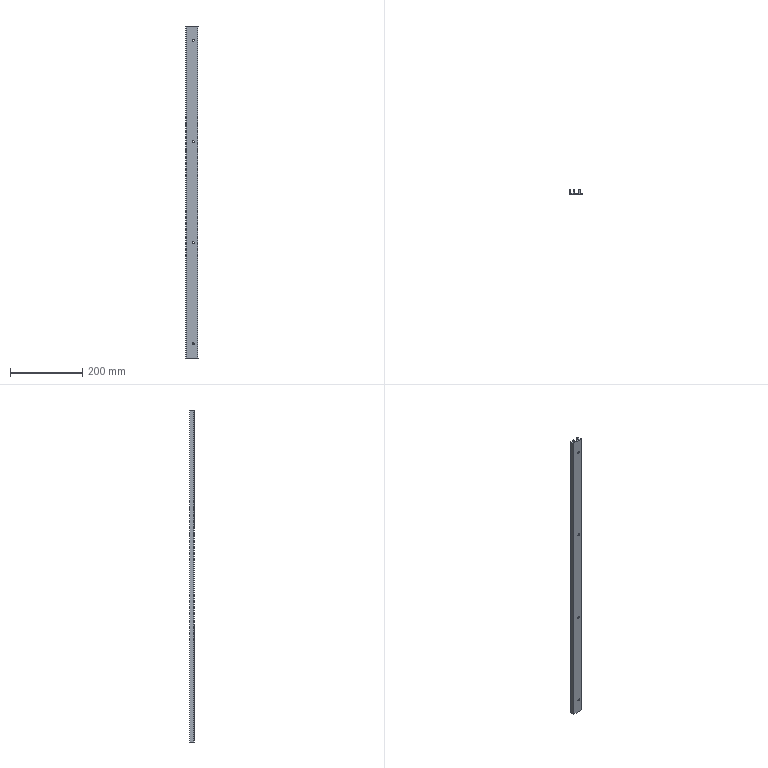Part | NX | features BREP 1 | 1 solid | 41 faces | box 33.5 x 13.5 x 919.5 mm | volume 171516 mm3 | cylinder 17 | plane 16 | cone 8 | commonest cylinder face diameters 5.5 x8 10.6 x4 4 x2 1.5 x1 2.5 x1 3 x1
STEP:
#1=CARTESIAN_POINT('',(22.75,0.45,-420.25));
#2=VERTEX_POINT('',#1);
#3=CARTESIAN_POINT('',(17.25,0.45,-420.25));
#4=VERTEX_POINT('',#3);
#5=CARTESIAN_POINT('',(20.,0.45,-420.25));
#6=DIRECTION('',(0.,1.,0.));
#7=DIRECTION('',(-1.,0.,0.));
#8=AXIS2_PLACEMENT_3D('',#5,#6,#7);
#9=CIRCLE('',#8,2.75);
#10=EDGE_CURVE('',#2,#4,#9,.T.);
#11=ORIENTED_EDGE('',*,*,#10,.F.);
#12=CARTESIAN_POINT('',(25.3,3.,-420.25));
#13=VERTEX_POINT('',#12);
#14=CARTESIAN_POINT('',(25.3,3.,-420.25));
#15=DIRECTION('',(0.7071,0.7071,0.));
#16=VECTOR('',#15,1000.);
#17=LINE('',#14,#16);
#18=EDGE_CURVE('',#2,#13,#17,.T.);
#19=ORIENTED_EDGE('',*,*,#18,.T.);
#20=CARTESIAN_POINT('',(24.5,3.,-423.05));
#21=VERTEX_POINT('',#20);
#22=CARTESIAN_POINT('',(20.,3.,-420.25));
#23=DIRECTION('',(0.,1.,0.));
#24=DIRECTION('',(-1.,0.,0.));
#25=AXIS2_PLACEMENT_3D('',#22,#23,#24);
#26=CIRCLE('',#25,5.3);
#27=EDGE_CURVE('',#13,#21,#26,.T.);
#28=ORIENTED_EDGE('',*,*,#27,.T.);
#29=CARTESIAN_POINT('',(14.7,3.,-420.25));
#30=VERTEX_POINT('',#29);
#31=CARTESIAN_POINT('',(20.,3.,-420.25));
#32=DIRECTION('',(0.,-1.,0.));
#33=DIRECTION('',(1.,0.,0.));
#34=AXIS2_PLACEMENT_3D('',#31,#32,#33);
#35=CIRCLE('',#34,5.3);
#36=EDGE_CURVE('',#30,#21,#35,.T.);
#37=ORIENTED_EDGE('',*,*,#36,.F.);
#38=CARTESIAN_POINT('',(14.7,3.,-420.25));
#39=DIRECTION('',(-0.7071,0.7071,0.));
#40=VECTOR('',#39,1000.);
#41=LINE('',#38,#40);
#42=EDGE_CURVE('',#4,#30,#41,.T.);
#43=ORIENTED_EDGE('',*,*,#42,.F.);
#44=EDGE_LOOP('',(#11,#19,#28,#37,#43));
#45=FACE_BOUND('',#44,.T.);
#46=CARTESIAN_POINT('',(20.,3.,-420.25));
#47=DIRECTION('',(0.,1.,0.));
#48=DIRECTION('',(-1.,0.,0.));
#49=AXIS2_PLACEMENT_3D('',#46,#47,#48);
#50=CONICAL_SURFACE('',#49,5.3,0.7854);
#51=ADVANCED_FACE('',(#45),#50,.F.);
#52=CARTESIAN_POINT('',(22.75,0.,-420.25));
#53=VERTEX_POINT('',#52);
#54=CARTESIAN_POINT('',(17.25,0.,-420.25));
#55=VERTEX_POINT('',#54);
#56=CARTESIAN_POINT('',(20.,0.,-420.25));
#57=DIRECTION('',(0.,1.,0.));
#58=DIRECTION('',(-1.,0.,0.));
#59=AXIS2_PLACEMENT_3D('',#56,#57,#58);
#60=CIRCLE('',#59,2.75);
#61=EDGE_CURVE('',#53,#55,#60,.T.);
#62=ORIENTED_EDGE('',*,*,#61,.F.);
#63=CARTESIAN_POINT('',(22.75,12.402,-420.25));
#64=DIRECTION('',(0.,1.,0.));
#65=VECTOR('',#64,1000.);
#66=LINE('',#63,#65);
#67=EDGE_CURVE('',#53,#2,#66,.T.);
#68=ORIENTED_EDGE('',*,*,#67,.T.);
#69=ORIENTED_EDGE('',*,*,#10,.T.);
#70=CARTESIAN_POINT('',(17.25,12.402,-420.25));
#71=DIRECTION('',(0.,1.,0.));
#72=VECTOR('',#71,1000.);
#73=LINE('',#70,#72);
#74=EDGE_CURVE('',#55,#4,#73,.T.);
#75=ORIENTED_EDGE('',*,*,#74,.F.);
#76=EDGE_LOOP('',(#62,#68,#69,#75));
#77=FACE_BOUND('',#76,.T.);
#78=CARTESIAN_POINT('',(20.,12.402,-420.25));
#79=DIRECTION('',(0.,1.,0.));
#80=DIRECTION('',(-1.,0.,0.));
#81=AXIS2_PLACEMENT_3D('',#78,#79,#80);
#82=CYLINDRICAL_SURFACE('',#81,2.75);
#83=ADVANCED_FACE('',(#77),#82,.F.);
#84=CARTESIAN_POINT('',(22.75,0.45,-140.25));
#85=VERTEX_POINT('',#84);
#86=CARTESIAN_POINT('',(17.25,0.45,-140.25));
#87=VERTEX_POINT('',#86);
#88=CARTESIAN_POINT('',(20.,0.45,-140.25));
#89=DIRECTION('',(0.,1.,0.));
#90=DIRECTION('',(-1.,0.,0.));
#91=AXIS2_PLACEMENT_3D('',#88,#89,#90);
#92=CIRCLE('',#91,2.75);
#93=EDGE_CURVE('',#85,#87,#92,.T.);
#94=ORIENTED_EDGE('',*,*,#93,.F.);
#95=CARTESIAN_POINT('',(25.3,3.,-140.25));
#96=VERTEX_POINT('',#95);
#97=CARTESIAN_POINT('',(25.3,3.,-140.25));
#98=DIRECTION('',(0.7071,0.7071,0.));
#99=VECTOR('',#98,1000.);
#100=LINE('',#97,#99);
#101=EDGE_CURVE('',#85,#96,#100,.T.);
#102=ORIENTED_EDGE('',*,*,#101,.T.);
#103=CARTESIAN_POINT('',(24.5,3.,-143.05));
#104=VERTEX_POINT('',#103);
#105=CARTESIAN_POINT('',(20.,3.,-140.25));
#106=DIRECTION('',(0.,1.,0.));
#107=DIRECTION('',(-1.,0.,0.));
#108=AXIS2_PLACEMENT_3D('',#105,#106,#107);
#109=CIRCLE('',#108,5.3);
#110=EDGE_CURVE('',#96,#104,#109,.T.);
#111=ORIENTED_EDGE('',*,*,#110,.T.);
#112=CARTESIAN_POINT('',(14.7,3.,-140.25));
#113=VERTEX_POINT('',#112);
#114=CARTESIAN_POINT('',(20.,3.,-140.25));
#115=DIRECTION('',(0.,-1.,0.));
#116=DIRECTION('',(1.,0.,0.));
#117=AXIS2_PLACEMENT_3D('',#114,#115,#116);
#118=CIRCLE('',#117,5.3);
#119=EDGE_CURVE('',#113,#104,#118,.T.);
#120=ORIENTED_EDGE('',*,*,#119,.F.);
#121=CARTESIAN_POINT('',(14.7,3.,-140.25));
#122=DIRECTION('',(-0.7071,0.7071,0.));
#123=VECTOR('',#122,1000.);
#124=LINE('',#121,#123);
#125=EDGE_CURVE('',#87,#113,#124,.T.);
#126=ORIENTED_EDGE('',*,*,#125,.F.);
#127=EDGE_LOOP('',(#94,#102,#111,#120,#126));
#128=FACE_BOUND('',#127,.T.);
#129=CARTESIAN_POINT('',(20.,3.,-140.25));
#130=DIRECTION('',(0.,1.,0.));
#131=DIRECTION('',(-1.,0.,0.));
#132=AXIS2_PLACEMENT_3D('',#129,#130,#131);
#133=CONICAL_SURFACE('',#132,5.3,0.7854);
#134=ADVANCED_FACE('',(#128),#133,.F.);
#135=CARTESIAN_POINT('',(22.75,0.,-140.25));
#136=VERTEX_POINT('',#135);
#137=CARTESIAN_POINT('',(17.25,0.,-140.25));
#138=VERTEX_POINT('',#137);
#139=CARTESIAN_POINT('',(20.,0.,-140.25));
#140=DIRECTION('',(0.,1.,0.));
#141=DIRECTION('',(-1.,0.,0.));
#142=AXIS2_PLACEMENT_3D('',#139,#140,#141);
#143=CIRCLE('',#142,2.75);
#144=EDGE_CURVE('',#136,#138,#143,.T.);
#145=ORIENTED_EDGE('',*,*,#144,.F.);
#146=CARTESIAN_POINT('',(22.75,12.402,-140.25));
#147=DIRECTION('',(0.,1.,0.));
#148=VECTOR('',#147,1000.);
#149=LINE('',#146,#148);
#150=EDGE_CURVE('',#136,#85,#149,.T.);
#151=ORIENTED_EDGE('',*,*,#150,.T.);
#152=ORIENTED_EDGE('',*,*,#93,.T.);
#153=CARTESIAN_POINT('',(17.25,12.402,-140.25));
#154=DIRECTION('',(0.,1.,0.));
#155=VECTOR('',#154,1000.);
#156=LINE('',#153,#155);
#157=EDGE_CURVE('',#138,#87,#156,.T.);
#158=ORIENTED_EDGE('',*,*,#157,.F.);
#159=EDGE_LOOP('',(#145,#151,#152,#158));
#160=FACE_BOUND('',#159,.T.);
#161=CARTESIAN_POINT('',(20.,12.402,-140.25));
#162=DIRECTION('',(0.,1.,0.));
#163=DIRECTION('',(-1.,0.,0.));
#164=AXIS2_PLACEMENT_3D('',#161,#162,#163);
#165=CYLINDRICAL_SURFACE('',#164,2.75);
#166=ADVANCED_FACE('',(#160),#165,.F.);
#167=CARTESIAN_POINT('',(22.75,0.45,139.75));
#168=VERTEX_POINT('',#167);
#169=CARTESIAN_POINT('',(17.25,0.45,139.75));
#170=VERTEX_POINT('',#169);
#171=CARTESIAN_POINT('',(20.,0.45,139.75));
#172=DIRECTION('',(0.,1.,0.));
#173=DIRECTION('',(-1.,0.,0.));
#174=AXIS2_PLACEMENT_3D('',#171,#172,#173);
#175=CIRCLE('',#174,2.75);
#176=EDGE_CURVE('',#168,#170,#175,.T.);
#177=ORIENTED_EDGE('',*,*,#176,.F.);
#178=CARTESIAN_POINT('',(25.3,3.,139.75));
#179=VERTEX_POINT('',#178);
#180=CARTESIAN_POINT('',(25.3,3.,139.75));
#181=DIRECTION('',(0.7071,0.7071,0.));
#182=VECTOR('',#181,1000.);
#183=LINE('',#180,#182);
#184=EDGE_CURVE('',#168,#179,#183,.T.);
#185=ORIENTED_EDGE('',*,*,#184,.T.);
#186=CARTESIAN_POINT('',(24.5,3.,136.95));
#187=VERTEX_POINT('',#186);
#188=CARTESIAN_POINT('',(20.,3.,139.75));
#189=DIRECTION('',(0.,1.,0.));
#190=DIRECTION('',(-1.,0.,0.));
#191=AXIS2_PLACEMENT_3D('',#188,#189,#190);
#192=CIRCLE('',#191,5.3);
#193=EDGE_CURVE('',#179,#187,#192,.T.);
#194=ORIENTED_EDGE('',*,*,#193,.T.);
#195=CARTESIAN_POINT('',(14.7,3.,139.75));
#196=VERTEX_POINT('',#195);
#197=CARTESIAN_POINT('',(20.,3.,139.75));
#198=DIRECTION('',(0.,-1.,0.));
#199=DIRECTION('',(1.,0.,0.));
#200=AXIS2_PLACEMENT_3D('',#197,#198,#199);
#201=CIRCLE('',#200,5.3);
#202=EDGE_CURVE('',#196,#187,#201,.T.);
#203=ORIENTED_EDGE('',*,*,#202,.F.);
#204=CARTESIAN_POINT('',(14.7,3.,139.75));
#205=DIRECTION('',(-0.7071,0.7071,0.));
#206=VECTOR('',#205,1000.);
#207=LINE('',#204,#206);
#208=EDGE_CURVE('',#170,#196,#207,.T.);
#209=ORIENTED_EDGE('',*,*,#208,.F.);
#210=EDGE_LOOP('',(#177,#185,#194,#203,#209));
#211=FACE_BOUND('',#210,.T.);
#212=CARTESIAN_POINT('',(20.,3.,139.75));
#213=DIRECTION('',(0.,1.,0.));
#214=DIRECTION('',(-1.,0.,0.));
#215=AXIS2_PLACEMENT_3D('',#212,#213,#214);
#216=CONICAL_SURFACE('',#215,5.3,0.7854);
#217=ADVANCED_FACE('',(#211),#216,.F.);
#218=CARTESIAN_POINT('',(22.75,0.,139.75));
#219=VERTEX_POINT('',#218);
#220=CARTESIAN_POINT('',(17.25,0.,139.75));
#221=VERTEX_POINT('',#220);
#222=CARTESIAN_POINT('',(20.,0.,139.75));
#223=DIRECTION('',(0.,1.,0.));
#224=DIRECTION('',(-1.,0.,0.));
#225=AXIS2_PLACEMENT_3D('',#222,#223,#224);
#226=CIRCLE('',#225,2.75);
#227=EDGE_CURVE('',#219,#221,#226,.T.);
#228=ORIENTED_EDGE('',*,*,#227,.F.);
#229=CARTESIAN_POINT('',(22.75,12.402,139.75));
#230=DIRECTION('',(0.,1.,0.));
#231=VECTOR('',#230,1000.);
#232=LINE('',#229,#231);
#233=EDGE_CURVE('',#219,#168,#232,.T.);
#234=ORIENTED_EDGE('',*,*,#233,.T.);
#235=ORIENTED_EDGE('',*,*,#176,.T.);
#236=CARTESIAN_POINT('',(17.25,12.402,139.75));
#237=DIRECTION('',(0.,1.,0.));
#238=VECTOR('',#237,1000.);
#239=LINE('',#236,#238);
#240=EDGE_CURVE('',#221,#170,#239,.T.);
#241=ORIENTED_EDGE('',*,*,#240,.F.);
#242=EDGE_LOOP('',(#228,#234,#235,#241));
#243=FACE_BOUND('',#242,.T.);
#244=CARTESIAN_POINT('',(20.,12.402,139.75));
#245=DIRECTION('',(0.,1.,0.));
#246=DIRECTION('',(-1.,0.,0.));
#247=AXIS2_PLACEMENT_3D('',#244,#245,#246);
#248=CYLINDRICAL_SURFACE('',#247,2.75);
#249=ADVANCED_FACE('',(#243),#248,.F.);
#250=CARTESIAN_POINT('',(22.75,0.45,419.75));
#251=VERTEX_POINT('',#250);
#252=CARTESIAN_POINT('',(17.25,0.45,419.75));
#253=VERTEX_POINT('',#252);
#254=CARTESIAN_POINT('',(20.,0.45,419.75));
#255=DIRECTION('',(0.,1.,0.));
#256=DIRECTION('',(-1.,0.,0.));
#257=AXIS2_PLACEMENT_3D('',#254,#255,#256);
#258=CIRCLE('',#257,2.75);
#259=EDGE_CURVE('',#251,#253,#258,.T.);
#260=ORIENTED_EDGE('',*,*,#259,.F.);
#261=CARTESIAN_POINT('',(25.3,3.,419.75));
#262=VERTEX_POINT('',#261);
#263=CARTESIAN_POINT('',(25.3,3.,419.75));
#264=DIRECTION('',(0.7071,0.7071,0.));
#265=VECTOR('',#264,1000.);
#266=LINE('',#263,#265);
#267=EDGE_CURVE('',#251,#262,#266,.T.);
#268=ORIENTED_EDGE('',*,*,#267,.T.);
#269=CARTESIAN_POINT('',(24.5,3.,416.95));
#270=VERTEX_POINT('',#269);
#271=CARTESIAN_POINT('',(20.,3.,419.75));
#272=DIRECTION('',(0.,1.,0.));
#273=DIRECTION('',(-1.,0.,0.));
#274=AXIS2_PLACEMENT_3D('',#271,#272,#273);
#275=CIRCLE('',#274,5.3);
#276=EDGE_CURVE('',#262,#270,#275,.T.);
#277=ORIENTED_EDGE('',*,*,#276,.T.);
#278=CARTESIAN_POINT('',(14.7,3.,419.75));
#279=VERTEX_POINT('',#278);
#280=CARTESIAN_POINT('',(20.,3.,419.75));
#281=DIRECTION('',(0.,-1.,0.));
#282=DIRECTION('',(1.,0.,0.));
#283=AXIS2_PLACEMENT_3D('',#280,#281,#282);
#284=CIRCLE('',#283,5.3);
#285=EDGE_CURVE('',#279,#270,#284,.T.);
#286=ORIENTED_EDGE('',*,*,#285,.F.);
#287=CARTESIAN_POINT('',(14.7,3.,419.75));
#288=DIRECTION('',(-0.7071,0.7071,0.));
#289=VECTOR('',#288,1000.);
#290=LINE('',#287,#289);
#291=EDGE_CURVE('',#253,#279,#290,.T.);
#292=ORIENTED_EDGE('',*,*,#291,.F.);
#293=EDGE_LOOP('',(#260,#268,#277,#286,#292));
#294=FACE_BOUND('',#293,.T.);
#295=CARTESIAN_POINT('',(20.,3.,419.75));
#296=DIRECTION('',(0.,1.,0.));
#297=DIRECTION('',(-1.,0.,0.));
#298=AXIS2_PLACEMENT_3D('',#295,#296,#297);
#299=CONICAL_SURFACE('',#298,5.3,0.7854);
#300=ADVANCED_FACE('',(#294),#299,.F.);
#301=CARTESIAN_POINT('',(22.75,0.,419.75));
#302=VERTEX_POINT('',#301);
#303=CARTESIAN_POINT('',(17.25,0.,419.75));
#304=VERTEX_POINT('',#303);
#305=CARTESIAN_POINT('',(20.,0.,419.75));
#306=DIRECTION('',(0.,1.,0.));
#307=DIRECTION('',(-1.,0.,0.));
#308=AXIS2_PLACEMENT_3D('',#305,#306,#307);
#309=CIRCLE('',#308,2.75);
#310=EDGE_CURVE('',#302,#304,#309,.T.);
#311=ORIENTED_EDGE('',*,*,#310,.F.);
#312=CARTESIAN_POINT('',(22.75,12.402,419.75));
#313=DIRECTION('',(0.,1.,0.));
#314=VECTOR('',#313,1000.);
#315=LINE('',#312,#314);
#316=EDGE_CURVE('',#302,#251,#315,.T.);
#317=ORIENTED_EDGE('',*,*,#316,.T.);
#318=ORIENTED_EDGE('',*,*,#259,.T.);
#319=CARTESIAN_POINT('',(17.25,12.402,419.75));
#320=DIRECTION('',(0.,1.,0.));
#321=VECTOR('',#320,1000.);
#322=LINE('',#319,#321);
#323=EDGE_CURVE('',#304,#253,#322,.T.);
#324=ORIENTED_EDGE('',*,*,#323,.F.);
#325=EDGE_LOOP('',(#311,#317,#318,#324));
#326=FACE_BOUND('',#325,.T.);
#327=CARTESIAN_POINT('',(20.,12.402,419.75));
#328=DIRECTION('',(0.,1.,0.));
#329=DIRECTION('',(-1.,0.,0.));
#330=AXIS2_PLACEMENT_3D('',#327,#328,#329);
#331=CYLINDRICAL_SURFACE('',#330,2.75);
#332=ADVANCED_FACE('',(#326),#331,.F.);
#333=CARTESIAN_POINT('',(24.5,3.,-459.75));
#334=VERTEX_POINT('',#333);
#335=CARTESIAN_POINT('',(24.5,3.,459.75));
#336=DIRECTION('',(0.,0.,-1.));
#337=VECTOR('',#336,1000.);
#338=LINE('',#335,#337);
#339=EDGE_CURVE('',#21,#334,#338,.T.);
#340=ORIENTED_EDGE('',*,*,#339,.F.);
#341=CARTESIAN_POINT('',(24.5,10.5,-423.05));
#342=VERTEX_POINT('',#341);
#343=CARTESIAN_POINT('',(24.5,12.402,-423.05));
#344=DIRECTION('',(0.,1.,0.));
#345=VECTOR('',#344,1000.);
#346=LINE('',#343,#345);
#347=EDGE_CURVE('',#21,#342,#346,.T.);
#348=ORIENTED_EDGE('',*,*,#347,.T.);
#349=CARTESIAN_POINT('',(24.5,10.5,-459.75));
#350=VERTEX_POINT('',#349);
#351=CARTESIAN_POINT('',(24.5,10.5,459.75));
#352=DIRECTION('',(0.,0.,-1.));
#353=VECTOR('',#352,1000.);
#354=LINE('',#351,#353);
#355=EDGE_CURVE('',#342,#350,#354,.T.);
#356=ORIENTED_EDGE('',*,*,#355,.T.);
#357=CARTESIAN_POINT('',(24.5,3.,-459.75));
#358=DIRECTION('',(0.,-1.,0.));
#359=VECTOR('',#358,1000.);
#360=LINE('',#357,#359);
#361=EDGE_CURVE('',#350,#334,#360,.T.);
#362=ORIENTED_EDGE('',*,*,#361,.T.);
#363=EDGE_LOOP('',(#340,#348,#356,#362));
#364=FACE_BOUND('',#363,.T.);
#365=CARTESIAN_POINT('',(24.5,3.,459.75));
#366=DIRECTION('',(1.,0.,0.));
#367=DIRECTION('',(0.,1.,0.));
#368=AXIS2_PLACEMENT_3D('',#365,#366,#367);
#369=PLANE('',#368);
#370=ADVANCED_FACE('',(#364),#369,.F.);
#371=CARTESIAN_POINT('',(24.5,10.5,-143.05));
#372=VERTEX_POINT('',#371);
#373=CARTESIAN_POINT('',(24.5,10.5,-417.45));
#374=VERTEX_POINT('',#373);
#375=CARTESIAN_POINT('',(24.5,10.5,459.75));
#376=DIRECTION('',(0.,0.,-1.));
#377=VECTOR('',#376,1000.);
#378=LINE('',#375,#377);
#379=EDGE_CURVE('',#372,#374,#378,.T.);
#380=ORIENTED_EDGE('',*,*,#379,.T.);
#381=CARTESIAN_POINT('',(24.5,3.,-417.45));
#382=VERTEX_POINT('',#381);
#383=CARTESIAN_POINT('',(24.5,12.402,-417.45));
#384=DIRECTION('',(0.,-1.,0.));
#385=VECTOR('',#384,1000.);
#386=LINE('',#383,#385);
#387=EDGE_CURVE('',#374,#382,#386,.T.);
#388=ORIENTED_EDGE('',*,*,#387,.T.);
#389=CARTESIAN_POINT('',(24.5,3.,459.75));
#390=DIRECTION('',(0.,0.,-1.));
#391=VECTOR('',#390,1000.);
#392=LINE('',#389,#391);
#393=EDGE_CURVE('',#104,#382,#392,.T.);
#394=ORIENTED_EDGE('',*,*,#393,.F.);
#395=CARTESIAN_POINT('',(24.5,12.402,-143.05));
#396=DIRECTION('',(0.,1.,0.));
#397=VECTOR('',#396,1000.);
#398=LINE('',#395,#397);
#399=EDGE_CURVE('',#104,#372,#398,.T.);
#400=ORIENTED_EDGE('',*,*,#399,.T.);
#401=EDGE_LOOP('',(#380,#388,#394,#400));
#402=FACE_BOUND('',#401,.T.);
#403=CARTESIAN_POINT('',(24.5,3.,459.75));
#404=DIRECTION('',(1.,0.,0.));
#405=DIRECTION('',(0.,1.,0.));
#406=AXIS2_PLACEMENT_3D('',#403,#404,#405);
#407=PLANE('',#406);
#408=ADVANCED_FACE('',(#402),#407,.F.);
#409=CARTESIAN_POINT('',(24.5,10.5,136.95));
#410=VERTEX_POINT('',#409);
#411=CARTESIAN_POINT('',(24.5,10.5,-137.45));
#412=VERTEX_POINT('',#411);
#413=CARTESIAN_POINT('',(24.5,10.5,459.75));
#414=DIRECTION('',(0.,0.,-1.));
#415=VECTOR('',#414,1000.);
#416=LINE('',#413,#415);
#417=EDGE_CURVE('',#410,#412,#416,.T.);
#418=ORIENTED_EDGE('',*,*,#417,.T.);
#419=CARTESIAN_POINT('',(24.5,3.,-137.45));
#420=VERTEX_POINT('',#419);
#421=CARTESIAN_POINT('',(24.5,12.402,-137.45));
#422=DIRECTION('',(0.,-1.,0.));
#423=VECTOR('',#422,1000.);
#424=LINE('',#421,#423);
#425=EDGE_CURVE('',#412,#420,#424,.T.);
#426=ORIENTED_EDGE('',*,*,#425,.T.);
#427=CARTESIAN_POINT('',(24.5,3.,459.75));
#428=DIRECTION('',(0.,0.,-1.));
#429=VECTOR('',#428,1000.);
#430=LINE('',#427,#429);
#431=EDGE_CURVE('',#187,#420,#430,.T.);
#432=ORIENTED_EDGE('',*,*,#431,.F.);
#433=CARTESIAN_POINT('',(24.5,12.402,136.95));
#434=DIRECTION('',(0.,1.,0.));
#435=VECTOR('',#434,1000.);
#436=LINE('',#433,#435);
#437=EDGE_CURVE('',#187,#410,#436,.T.);
#438=ORIENTED_EDGE('',*,*,#437,.T.);
#439=EDGE_LOOP('',(#418,#426,#432,#438));
#440=FACE_BOUND('',#439,.T.);
#441=CARTESIAN_POINT('',(24.5,3.,459.75));
#442=DIRECTION('',(1.,0.,0.));
#443=DIRECTION('',(0.,1.,0.));
#444=AXIS2_PLACEMENT_3D('',#441,#442,#443);
#445=PLANE('',#444);
#446=ADVANCED_FACE('',(#440),#445,.F.);
#447=CARTESIAN_POINT('',(24.5,10.5,416.95));
#448=VERTEX_POINT('',#447);
#449=CARTESIAN_POINT('',(24.5,10.5,142.55));
#450=VERTEX_POINT('',#449);
#451=CARTESIAN_POINT('',(24.5,10.5,459.75));
#452=DIRECTION('',(0.,0.,-1.));
#453=VECTOR('',#452,1000.);
#454=LINE('',#451,#453);
#455=EDGE_CURVE('',#448,#450,#454,.T.);
#456=ORIENTED_EDGE('',*,*,#455,.T.);
#457=CARTESIAN_POINT('',(24.5,3.,142.55));
#458=VERTEX_POINT('',#457);
#459=CARTESIAN_POINT('',(24.5,12.402,142.55));
#460=DIRECTION('',(0.,-1.,0.));
#461=VECTOR('',#460,1000.);
#462=LINE('',#459,#461);
#463=EDGE_CURVE('',#450,#458,#462,.T.);
#464=ORIENTED_EDGE('',*,*,#463,.T.);
#465=CARTESIAN_POINT('',(24.5,3.,459.75));
#466=DIRECTION('',(0.,0.,-1.));
#467=VECTOR('',#466,1000.);
#468=LINE('',#465,#467);
#469=EDGE_CURVE('',#270,#458,#468,.T.);
#470=ORIENTED_EDGE('',*,*,#469,.F.);
#471=CARTESIAN_POINT('',(24.5,12.402,416.95));
#472=DIRECTION('',(0.,1.,0.));
#473=VECTOR('',#472,1000.);
#474=LINE('',#471,#473);
#475=EDGE_CURVE('',#270,#448,#474,.T.);
#476=ORIENTED_EDGE('',*,*,#475,.T.);
#477=EDGE_LOOP('',(#456,#464,#470,#476));
#478=FACE_BOUND('',#477,.T.);
#479=CARTESIAN_POINT('',(24.5,3.,459.75));
#480=DIRECTION('',(1.,0.,0.));
#481=DIRECTION('',(0.,1.,0.));
#482=AXIS2_PLACEMENT_3D('',#479,#480,#481);
#483=PLANE('',#482);
#484=ADVANCED_FACE('',(#478),#483,.F.);
#485=CARTESIAN_POINT('',(0.,1.25,-459.75));
#486=VERTEX_POINT('',#485);
#487=CARTESIAN_POINT('',(1.25,0.,-459.75));
#488=VERTEX_POINT('',#487);
#489=CARTESIAN_POINT('',(1.25,1.25,-459.75));
#490=DIRECTION('',(0.,0.,1.));
#491=DIRECTION('',(1.,0.,0.));
#492=AXIS2_PLACEMENT_3D('',#489,#490,#491);
#493=CIRCLE('',#492,1.25);
#494=EDGE_CURVE('',#486,#488,#493,.T.);
#495=ORIENTED_EDGE('',*,*,#494,.T.);
#496=CARTESIAN_POINT('',(1.25,0.,459.75));
#497=VERTEX_POINT('',#496);
#498=CARTESIAN_POINT('',(1.25,0.,459.75));
#499=DIRECTION('',(0.,0.,-1.));
#500=VECTOR('',#499,1000.);
#501=LINE('',#498,#500);
#502=EDGE_CURVE('',#497,#488,#501,.T.);
#503=ORIENTED_EDGE('',*,*,#502,.F.);
#504=CARTESIAN_POINT('',(0.,1.25,459.75));
#505=VERTEX_POINT('',#504);
#506=CARTESIAN_POINT('',(1.25,1.25,459.75));
#507=DIRECTION('',(0.,0.,1.));
#508=DIRECTION('',(1.,0.,0.));
#509=AXIS2_PLACEMENT_3D('',#506,#507,#508);
#510=CIRCLE('',#509,1.25);
#511=EDGE_CURVE('',#505,#497,#510,.T.);
#512=ORIENTED_EDGE('',*,*,#511,.F.);
#513=CARTESIAN_POINT('',(0.,1.25,459.75));
#514=DIRECTION('',(0.,0.,-1.));
#515=VECTOR('',#514,1000.);
#516=LINE('',#513,#515);
#517=EDGE_CURVE('',#505,#486,#516,.T.);
#518=ORIENTED_EDGE('',*,*,#517,.T.);
#519=EDGE_LOOP('',(#495,#503,#512,#518));
#520=FACE_BOUND('',#519,.T.);
#521=CARTESIAN_POINT('',(1.25,1.25,459.75));
#522=DIRECTION('',(0.,0.,-1.));
#523=DIRECTION('',(-1.,0.,0.));
#524=AXIS2_PLACEMENT_3D('',#521,#522,#523);
#525=CYLINDRICAL_SURFACE('',#524,1.25);
#526=ADVANCED_FACE('',(#520),#525,.T.);
#527=CARTESIAN_POINT('',(32.,0.,-459.75));
#528=VERTEX_POINT('',#527);
#529=CARTESIAN_POINT('',(1.25,0.,-459.75));
#530=DIRECTION('',(1.,0.,0.));
#531=VECTOR('',#530,1000.);
#532=LINE('',#529,#531);
#533=EDGE_CURVE('',#488,#528,#532,.T.);
#534=ORIENTED_EDGE('',*,*,#533,.T.);
#535=CARTESIAN_POINT('',(32.,0.,459.75));
#536=VERTEX_POINT('',#535);
#537=CARTESIAN_POINT('',(32.,0.,459.75));
#538=DIRECTION('',(0.,0.,-1.));
#539=VECTOR('',#538,1000.);
#540=LINE('',#537,#539);
#541=EDGE_CURVE('',#536,#528,#540,.T.);
#542=ORIENTED_EDGE('',*,*,#541,.F.);
#543=CARTESIAN_POINT('',(1.25,0.,459.75));
#544=DIRECTION('',(1.,0.,0.));
#545=VECTOR('',#544,1000.);
#546=LINE('',#543,#545);
#547=EDGE_CURVE('',#497,#536,#546,.T.);
#548=ORIENTED_EDGE('',*,*,#547,.F.);
#549=ORIENTED_EDGE('',*,*,#502,.T.);
#550=EDGE_LOOP('',(#534,#542,#548,#549));
#551=FACE_BOUND('',#550,.T.);
#552=CARTESIAN_POINT('',(20.,0.,-420.25));
#553=DIRECTION('',(0.,1.,0.));
#554=DIRECTION('',(-1.,0.,0.));
#555=AXIS2_PLACEMENT_3D('',#552,#553,#554);
#556=CIRCLE('',#555,2.75);
#557=EDGE_CURVE('',#55,#53,#556,.T.);
#558=ORIENTED_EDGE('',*,*,#557,.T.);
#559=ORIENTED_EDGE('',*,*,#61,.T.);
#560=EDGE_LOOP('',(#558,#559));
#561=FACE_BOUND('',#560,.T.);
#562=CARTESIAN_POINT('',(20.,0.,-140.25));
#563=DIRECTION('',(0.,1.,0.));
#564=DIRECTION('',(-1.,0.,0.));
#565=AXIS2_PLACEMENT_3D('',#562,#563,#564);
#566=CIRCLE('',#565,2.75);
#567=EDGE_CURVE('',#138,#136,#566,.T.);
#568=ORIENTED_EDGE('',*,*,#567,.T.);
#569=ORIENTED_EDGE('',*,*,#144,.T.);
#570=EDGE_LOOP('',(#568,#569));
#571=FACE_BOUND('',#570,.T.);
#572=CARTESIAN_POINT('',(20.,0.,139.75));
#573=DIRECTION('',(0.,1.,0.));
#574=DIRECTION('',(-1.,0.,0.));
#575=AXIS2_PLACEMENT_3D('',#572,#573,#574);
#576=CIRCLE('',#575,2.75);
#577=EDGE_CURVE('',#221,#219,#576,.T.);
#578=ORIENTED_EDGE('',*,*,#577,.T.);
#579=ORIENTED_EDGE('',*,*,#227,.T.);
#580=EDGE_LOOP('',(#578,#579));
#581=FACE_BOUND('',#580,.T.);
#582=CARTESIAN_POINT('',(20.,0.,419.75));
#583=DIRECTION('',(0.,1.,0.));
#584=DIRECTION('',(-1.,0.,0.));
#585=AXIS2_PLACEMENT_3D('',#582,#583,#584);
#586=CIRCLE('',#585,2.75);
#587=EDGE_CURVE('',#304,#302,#586,.T.);
#588=ORIENTED_EDGE('',*,*,#587,.T.);
#589=ORIENTED_EDGE('',*,*,#310,.T.);
#590=EDGE_LOOP('',(#588,#589));
#591=FACE_BOUND('',#590,.T.);
#592=CARTESIAN_POINT('',(1.25,0.,459.75));
#593=DIRECTION('',(0.,1.,0.));
#594=DIRECTION('',(1.,0.,0.));
#595=AXIS2_PLACEMENT_3D('',#592,#593,#594);
#596=PLANE('',#595);
#597=ADVANCED_FACE('',(#551,#561,#571,#581,#591),#596,.F.);
#598=CARTESIAN_POINT('',(32.,3.,-459.75));
#599=VERTEX_POINT('',#598);
#600=CARTESIAN_POINT('',(32.,1.5,-459.75));
#601=DIRECTION('',(0.,0.,1.));
#602=DIRECTION('',(-1.,0.,0.));
#603=AXIS2_PLACEMENT_3D('',#600,#601,#602);
#604=CIRCLE('',#603,1.5);
#605=EDGE_CURVE('',#528,#599,#604,.T.);
#606=ORIENTED_EDGE('',*,*,#605,.T.);
#607=CARTESIAN_POINT('',(32.,3.,459.75));
#608=VERTEX_POINT('',#607);
#609=CARTESIAN_POINT('',(32.,3.,459.75));
#610=DIRECTION('',(0.,0.,-1.));
#611=VECTOR('',#610,1000.);
#612=LINE('',#609,#611);
#613=EDGE_CURVE('',#608,#599,#612,.T.);
#614=ORIENTED_EDGE('',*,*,#613,.F.);
#615=CARTESIAN_POINT('',(32.,1.5,459.75));
#616=DIRECTION('',(0.,0.,1.));
#617=DIRECTION('',(-1.,0.,0.));
#618=AXIS2_PLACEMENT_3D('',#615,#616,#617);
#619=CIRCLE('',#618,1.5);
#620=EDGE_CURVE('',#536,#608,#619,.T.);
#621=ORIENTED_EDGE('',*,*,#620,.F.);
#622=ORIENTED_EDGE('',*,*,#541,.T.);
#623=EDGE_LOOP('',(#606,#614,#621,#622));
#624=FACE_BOUND('',#623,.T.);
#625=CARTESIAN_POINT('',(32.,1.5,459.75));
#626=DIRECTION('',(0.,0.,-1.));
#627=DIRECTION('',(-1.,0.,0.));
#628=AXIS2_PLACEMENT_3D('',#625,#626,#627);
#629=CYLINDRICAL_SURFACE('',#628,1.5);
#630=ADVANCED_FACE('',(#624),#629,.T.);
#631=CARTESIAN_POINT('',(28.5,3.,-459.75));
#632=VERTEX_POINT('',#631);
#633=CARTESIAN_POINT('',(28.5,3.,-459.75));
#634=DIRECTION('',(-1.,0.,0.));
#635=VECTOR('',#634,1000.);
#636=LINE('',#633,#635);
#637=EDGE_CURVE('',#599,#632,#636,.T.);
#638=ORIENTED_EDGE('',*,*,#637,.T.);
#639=CARTESIAN_POINT('',(28.5,3.,459.75));
#640=VERTEX_POINT('',#639);
#641=CARTESIAN_POINT('',(28.5,3.,459.75));
#642=DIRECTION('',(0.,0.,-1.));
#643=VECTOR('',#642,1000.);
#644=LINE('',#641,#643);
#645=EDGE_CURVE('',#640,#632,#644,.T.);
#646=ORIENTED_EDGE('',*,*,#645,.F.);
#647=CARTESIAN_POINT('',(28.5,3.,459.75));
#648=DIRECTION('',(-1.,0.,0.));
#649=VECTOR('',#648,1000.);
#650=LINE('',#647,#649);
#651=EDGE_CURVE('',#608,#640,#650,.T.);
#652=ORIENTED_EDGE('',*,*,#651,.F.);
#653=ORIENTED_EDGE('',*,*,#613,.T.);
#654=EDGE_LOOP('',(#638,#646,#652,#653));
#655=FACE_BOUND('',#654,.T.);
#656=CARTESIAN_POINT('',(28.5,3.,459.75));
#657=DIRECTION('',(0.,-1.,0.));
#658=DIRECTION('',(0.,0.,-1.));
#659=AXIS2_PLACEMENT_3D('',#656,#657,#658);
#660=PLANE('',#659);
#661=ADVANCED_FACE('',(#655),#660,.F.);
#662=CARTESIAN_POINT('',(28.5,10.5,-459.75));
#663=VERTEX_POINT('',#662);
#664=CARTESIAN_POINT('',(28.5,10.5,-459.75));
#665=DIRECTION('',(0.,1.,0.));
#666=VECTOR('',#665,1000.);
#667=LINE('',#664,#666);
#668=EDGE_CURVE('',#632,#663,#667,.T.);
#669=ORIENTED_EDGE('',*,*,#668,.T.);
#670=CARTESIAN_POINT('',(28.5,10.5,459.75));
#671=VERTEX_POINT('',#670);
#672=CARTESIAN_POINT('',(28.5,10.5,459.75));
#673=DIRECTION('',(0.,0.,-1.));
#674=VECTOR('',#673,1000.);
#675=LINE('',#672,#674);
#676=EDGE_CURVE('',#671,#663,#675,.T.);
#677=ORIENTED_EDGE('',*,*,#676,.F.);
#678=CARTESIAN_POINT('',(28.5,10.5,459.75));
#679=DIRECTION('',(0.,1.,0.));
#680=VECTOR('',#679,1000.);
#681=LINE('',#678,#680);
#682=EDGE_CURVE('',#640,#671,#681,.T.);
#683=ORIENTED_EDGE('',*,*,#682,.F.);
#684=ORIENTED_EDGE('',*,*,#645,.T.);
#685=EDGE_LOOP('',(#669,#677,#683,#684));
#686=FACE_BOUND('',#685,.T.);
#687=CARTESIAN_POINT('',(28.5,10.5,459.75));
#688=DIRECTION('',(-1.,0.,0.));
#689=DIRECTION('',(0.,0.,1.));
#690=AXIS2_PLACEMENT_3D('',#687,#688,#689);
#691=PLANE('',#690);
#692=ADVANCED_FACE('',(#686),#691,.F.);
#693=ORIENTED_EDGE('',*,*,#355,.F.);
#694=CARTESIAN_POINT('',(24.5,10.5,-423.05));
#695=CARTESIAN_POINT('',(24.5,10.807,-423.05));
#696=CARTESIAN_POINT('',(24.662,11.403,-422.801));
#697=CARTESIAN_POINT('',(25.131,12.006,-421.793));
#698=CARTESIAN_POINT('',(25.412,12.162,-420.25));
#699=CARTESIAN_POINT('',(25.133,12.008,-418.711));
#700=CARTESIAN_POINT('',(24.662,11.404,-417.699));
#701=CARTESIAN_POINT('',(24.5,10.808,-417.45));
#702=CARTESIAN_POINT('',(24.5,10.5,-417.45));
#703=B_SPLINE_CURVE_WITH_KNOTS('',3,(#694,#695,#696,#697,#698,#699,#700,#701,#702),.UNSPECIFIED.,.F.,.F.,(4,1,1,1,1,1,4),(0.,0.125,0.25,0.5,0.75,0.875,1.),.UNSPECIFIED.);
#704=EDGE_CURVE('',#342,#374,#703,.T.);
#705=ORIENTED_EDGE('',*,*,#704,.T.);
#706=ORIENTED_EDGE('',*,*,#379,.F.);
#707=CARTESIAN_POINT('',(24.5,10.5,-143.05));
#708=CARTESIAN_POINT('',(24.5,10.807,-143.05));
#709=CARTESIAN_POINT('',(24.662,11.403,-142.801));
#710=CARTESIAN_POINT('',(25.131,12.006,-141.793));
#711=CARTESIAN_POINT('',(25.412,12.162,-140.25));
#712=CARTESIAN_POINT('',(25.133,12.008,-138.711));
#713=CARTESIAN_POINT('',(24.662,11.404,-137.699));
#714=CARTESIAN_POINT('',(24.5,10.808,-137.45));
#715=CARTESIAN_POINT('',(24.5,10.5,-137.45));
#716=B_SPLINE_CURVE_WITH_KNOTS('',3,(#707,#708,#709,#710,#711,#712,#713,#714,#715),.UNSPECIFIED.,.F.,.F.,(4,1,1,1,1,1,4),(0.,0.125,0.25,0.5,0.75,0.875,1.),.UNSPECIFIED.);
#717=EDGE_CURVE('',#372,#412,#716,.T.);
#718=ORIENTED_EDGE('',*,*,#717,.T.);
#719=ORIENTED_EDGE('',*,*,#417,.F.);
#720=CARTESIAN_POINT('',(24.5,10.5,136.95));
#721=CARTESIAN_POINT('',(24.5,10.807,136.95));
#722=CARTESIAN_POINT('',(24.662,11.403,137.199));
#723=CARTESIAN_POINT('',(25.131,12.006,138.207));
#724=CARTESIAN_POINT('',(25.412,12.162,139.75));
#725=CARTESIAN_POINT('',(25.133,12.008,141.289));
#726=CARTESIAN_POINT('',(24.662,11.404,142.301));
#727=CARTESIAN_POINT('',(24.5,10.808,142.55));
#728=CARTESIAN_POINT('',(24.5,10.5,142.55));
#729=B_SPLINE_CURVE_WITH_KNOTS('',3,(#720,#721,#722,#723,#724,#725,#726,#727,#728),.UNSPECIFIED.,.F.,.F.,(4,1,1,1,1,1,4),(0.,0.125,0.25,0.5,0.75,0.875,1.),.UNSPECIFIED.);
#730=EDGE_CURVE('',#410,#450,#729,.T.);
#731=ORIENTED_EDGE('',*,*,#730,.T.);
#732=ORIENTED_EDGE('',*,*,#455,.F.);
#733=CARTESIAN_POINT('',(24.5,10.5,422.55));
#734=VERTEX_POINT('',#733);
#735=CARTESIAN_POINT('',(24.5,10.5,416.95));
#736=CARTESIAN_POINT('',(24.5,10.807,416.95));
#737=CARTESIAN_POINT('',(24.662,11.403,417.199));
#738=CARTESIAN_POINT('',(25.131,12.006,418.207));
#739=CARTESIAN_POINT('',(25.412,12.162,419.75));
#740=CARTESIAN_POINT('',(25.133,12.008,421.289));
#741=CARTESIAN_POINT('',(24.662,11.404,422.301));
#742=CARTESIAN_POINT('',(24.5,10.808,422.55));
#743=CARTESIAN_POINT('',(24.5,10.5,422.55));
#744=B_SPLINE_CURVE_WITH_KNOTS('',3,(#735,#736,#737,#738,#739,#740,#741,#742,#743),.UNSPECIFIED.,.F.,.F.,(4,1,1,1,1,1,4),(0.,0.125,0.25,0.5,0.75,0.875,1.),.UNSPECIFIED.);
#745=EDGE_CURVE('',#448,#734,#744,.T.);
#746=ORIENTED_EDGE('',*,*,#745,.T.);
#747=CARTESIAN_POINT('',(24.5,10.5,459.75));
#748=VERTEX_POINT('',#747);
#749=CARTESIAN_POINT('',(24.5,10.5,459.75));
#750=DIRECTION('',(0.,0.,-1.));
#751=VECTOR('',#750,1000.);
#752=LINE('',#749,#751);
#753=EDGE_CURVE('',#748,#734,#752,.T.);
#754=ORIENTED_EDGE('',*,*,#753,.F.);
#755=CARTESIAN_POINT('',(26.5,10.5,459.75));
#756=DIRECTION('',(0.,0.,1.));
#757=DIRECTION('',(-1.,0.,0.));
#758=AXIS2_PLACEMENT_3D('',#755,#756,#757);
#759=CIRCLE('',#758,2.);
#760=EDGE_CURVE('',#671,#748,#759,.T.);
#761=ORIENTED_EDGE('',*,*,#760,.F.);
#762=ORIENTED_EDGE('',*,*,#676,.T.);
#763=CARTESIAN_POINT('',(26.5,10.5,-459.75));
#764=DIRECTION('',(0.,0.,1.));
#765=DIRECTION('',(-1.,0.,0.));
#766=AXIS2_PLACEMENT_3D('',#763,#764,#765);
#767=CIRCLE('',#766,2.);
#768=EDGE_CURVE('',#663,#350,#767,.T.);
#769=ORIENTED_EDGE('',*,*,#768,.T.);
#770=EDGE_LOOP('',(#693,#705,#706,#718,#719,#731,#732,#746,#754,#761,#762,#769));
#771=FACE_BOUND('',#770,.T.);
#772=CARTESIAN_POINT('',(26.5,10.5,459.75));
#773=DIRECTION('',(0.,0.,-1.));
#774=DIRECTION('',(-1.,0.,0.));
#775=AXIS2_PLACEMENT_3D('',#772,#773,#774);
#776=CYLINDRICAL_SURFACE('',#775,2.);
#777=ADVANCED_FACE('',(#771),#776,.T.);
#778=ORIENTED_EDGE('',*,*,#753,.T.);
#779=CARTESIAN_POINT('',(24.5,3.,422.55));
#780=VERTEX_POINT('',#779);
#781=CARTESIAN_POINT('',(24.5,12.402,422.55));
#782=DIRECTION('',(0.,-1.,0.));
#783=VECTOR('',#782,1000.);
#784=LINE('',#781,#783);
#785=EDGE_CURVE('',#734,#780,#784,.T.);
#786=ORIENTED_EDGE('',*,*,#785,.T.);
#787=CARTESIAN_POINT('',(24.5,3.,459.75));
#788=VERTEX_POINT('',#787);
#789=CARTESIAN_POINT('',(24.5,3.,459.75));
#790=DIRECTION('',(0.,0.,-1.));
#791=VECTOR('',#790,1000.);
#792=LINE('',#789,#791);
#793=EDGE_CURVE('',#788,#780,#792,.T.);
#794=ORIENTED_EDGE('',*,*,#793,.F.);
#795=CARTESIAN_POINT('',(24.5,3.,459.75));
#796=DIRECTION('',(0.,-1.,0.));
#797=VECTOR('',#796,1000.);
#798=LINE('',#795,#797);
#799=EDGE_CURVE('',#748,#788,#798,.T.);
#800=ORIENTED_EDGE('',*,*,#799,.F.);
#801=EDGE_LOOP('',(#778,#786,#794,#800));
#802=FACE_BOUND('',#801,.T.);
#803=CARTESIAN_POINT('',(24.5,3.,459.75));
#804=DIRECTION('',(1.,0.,0.));
#805=DIRECTION('',(0.,1.,0.));
#806=AXIS2_PLACEMENT_3D('',#803,#804,#805);
#807=PLANE('',#806);
#808=ADVANCED_FACE('',(#802),#807,.F.);
#809=ORIENTED_EDGE('',*,*,#393,.T.);
#810=CARTESIAN_POINT('',(20.,3.,-420.25));
#811=DIRECTION('',(0.,-1.,0.));
#812=DIRECTION('',(1.,0.,0.));
#813=AXIS2_PLACEMENT_3D('',#810,#811,#812);
#814=CIRCLE('',#813,5.3);
#815=EDGE_CURVE('',#382,#30,#814,.T.);
#816=ORIENTED_EDGE('',*,*,#815,.T.);
#817=ORIENTED_EDGE('',*,*,#36,.T.);
#818=ORIENTED_EDGE('',*,*,#339,.T.);
#819=CARTESIAN_POINT('',(12.5,3.,-459.75));
#820=VERTEX_POINT('',#819);
#821=CARTESIAN_POINT('',(12.5,3.,-459.75));
#822=DIRECTION('',(-1.,0.,0.));
#823=VECTOR('',#822,1000.);
#824=LINE('',#821,#823);
#825=EDGE_CURVE('',#334,#820,#824,.T.);
#826=ORIENTED_EDGE('',*,*,#825,.T.);
#827=CARTESIAN_POINT('',(12.5,3.,459.75));
#828=VERTEX_POINT('',#827);
#829=CARTESIAN_POINT('',(12.5,3.,459.75));
#830=DIRECTION('',(0.,0.,-1.));
#831=VECTOR('',#830,1000.);
#832=LINE('',#829,#831);
#833=EDGE_CURVE('',#828,#820,#832,.T.);
#834=ORIENTED_EDGE('',*,*,#833,.F.);
#835=CARTESIAN_POINT('',(12.5,3.,459.75));
#836=DIRECTION('',(-1.,0.,0.));
#837=VECTOR('',#836,1000.);
#838=LINE('',#835,#837);
#839=EDGE_CURVE('',#788,#828,#838,.T.);
#840=ORIENTED_EDGE('',*,*,#839,.F.);
#841=ORIENTED_EDGE('',*,*,#793,.T.);
#842=CARTESIAN_POINT('',(20.,3.,419.75));
#843=DIRECTION('',(0.,-1.,0.));
#844=DIRECTION('',(1.,0.,0.));
#845=AXIS2_PLACEMENT_3D('',#842,#843,#844);
#846=CIRCLE('',#845,5.3);
#847=EDGE_CURVE('',#780,#279,#846,.T.);
#848=ORIENTED_EDGE('',*,*,#847,.T.);
#849=ORIENTED_EDGE('',*,*,#285,.T.);
#850=ORIENTED_EDGE('',*,*,#469,.T.);
#851=CARTESIAN_POINT('',(20.,3.,139.75));
#852=DIRECTION('',(0.,-1.,0.));
#853=DIRECTION('',(1.,0.,0.));
#854=AXIS2_PLACEMENT_3D('',#851,#852,#853);
#855=CIRCLE('',#854,5.3);
#856=EDGE_CURVE('',#458,#196,#855,.T.);
#857=ORIENTED_EDGE('',*,*,#856,.T.);
#858=ORIENTED_EDGE('',*,*,#202,.T.);
#859=ORIENTED_EDGE('',*,*,#431,.T.);
#860=CARTESIAN_POINT('',(20.,3.,-140.25));
#861=DIRECTION('',(0.,-1.,0.));
#862=DIRECTION('',(1.,0.,0.));
#863=AXIS2_PLACEMENT_3D('',#860,#861,#862);
#864=CIRCLE('',#863,5.3);
#865=EDGE_CURVE('',#420,#113,#864,.T.);
#866=ORIENTED_EDGE('',*,*,#865,.T.);
#867=ORIENTED_EDGE('',*,*,#119,.T.);
#868=EDGE_LOOP('',(#809,#816,#817,#818,#826,#834,#840,#841,#848,#849,#850,#857,#858,#859,#866,#867));
#869=FACE_BOUND('',#868,.T.);
#870=CARTESIAN_POINT('',(12.5,3.,459.75));
#871=DIRECTION('',(0.,-1.,0.));
#872=DIRECTION('',(0.,0.,-1.));
#873=AXIS2_PLACEMENT_3D('',#870,#871,#872);
#874=PLANE('',#873);
#875=ADVANCED_FACE('',(#869),#874,.F.);
#876=CARTESIAN_POINT('',(12.5,10.5,-459.75));
#877=VERTEX_POINT('',#876);
#878=CARTESIAN_POINT('',(12.5,10.5,-459.75));
#879=DIRECTION('',(0.,1.,0.));
#880=VECTOR('',#879,1000.);
#881=LINE('',#878,#880);
#882=EDGE_CURVE('',#820,#877,#881,.T.);
#883=ORIENTED_EDGE('',*,*,#882,.T.);
#884=CARTESIAN_POINT('',(12.5,10.5,459.75));
#885=VERTEX_POINT('',#884);
#886=CARTESIAN_POINT('',(12.5,10.5,459.75));
#887=DIRECTION('',(0.,0.,-1.));
#888=VECTOR('',#887,1000.);
#889=LINE('',#886,#888);
#890=EDGE_CURVE('',#885,#877,#889,.T.);
#891=ORIENTED_EDGE('',*,*,#890,.F.);
#892=CARTESIAN_POINT('',(12.5,10.5,459.75));
#893=DIRECTION('',(0.,1.,0.));
#894=VECTOR('',#893,1000.);
#895=LINE('',#892,#894);
#896=EDGE_CURVE('',#828,#885,#895,.T.);
#897=ORIENTED_EDGE('',*,*,#896,.F.);
#898=ORIENTED_EDGE('',*,*,#833,.T.);
#899=EDGE_LOOP('',(#883,#891,#897,#898));
#900=FACE_BOUND('',#899,.T.);
#901=CARTESIAN_POINT('',(12.5,10.5,459.75));
#902=DIRECTION('',(-1.,0.,0.));
#903=DIRECTION('',(0.,1.,0.));
#904=AXIS2_PLACEMENT_3D('',#901,#902,#903);
#905=PLANE('',#904);
#906=ADVANCED_FACE('',(#900),#905,.F.);
#907=CARTESIAN_POINT('',(8.5,10.5,-459.75));
#908=VERTEX_POINT('',#907);
#909=CARTESIAN_POINT('',(10.5,10.5,-459.75));
#910=DIRECTION('',(0.,0.,1.));
#911=DIRECTION('',(1.,0.,0.));
#912=AXIS2_PLACEMENT_3D('',#909,#910,#911);
#913=CIRCLE('',#912,2.);
#914=EDGE_CURVE('',#877,#908,#913,.T.);
#915=ORIENTED_EDGE('',*,*,#914,.T.);
#916=CARTESIAN_POINT('',(8.5,10.5,459.75));
#917=VERTEX_POINT('',#916);
#918=CARTESIAN_POINT('',(8.5,10.5,459.75));
#919=DIRECTION('',(0.,0.,-1.));
#920=VECTOR('',#919,1000.);
#921=LINE('',#918,#920);
#922=EDGE_CURVE('',#917,#908,#921,.T.);
#923=ORIENTED_EDGE('',*,*,#922,.F.);
#924=CARTESIAN_POINT('',(10.5,10.5,459.75));
#925=DIRECTION('',(0.,0.,1.));
#926=DIRECTION('',(1.,0.,0.));
#927=AXIS2_PLACEMENT_3D('',#924,#925,#926);
#928=CIRCLE('',#927,2.);
#929=EDGE_CURVE('',#885,#917,#928,.T.);
#930=ORIENTED_EDGE('',*,*,#929,.F.);
#931=ORIENTED_EDGE('',*,*,#890,.T.);
#932=EDGE_LOOP('',(#915,#923,#930,#931));
#933=FACE_BOUND('',#932,.T.);
#934=CARTESIAN_POINT('',(10.5,10.5,459.75));
#935=DIRECTION('',(0.,0.,-1.));
#936=DIRECTION('',(-1.,0.,0.));
#937=AXIS2_PLACEMENT_3D('',#934,#935,#936);
#938=CYLINDRICAL_SURFACE('',#937,2.);
#939=ADVANCED_FACE('',(#933),#938,.T.);
#940=CARTESIAN_POINT('',(8.5,3.,-459.75));
#941=VERTEX_POINT('',#940);
#942=CARTESIAN_POINT('',(8.5,3.,-459.75));
#943=DIRECTION('',(0.,-1.,0.));
#944=VECTOR('',#943,1000.);
#945=LINE('',#942,#944);
#946=EDGE_CURVE('',#908,#941,#945,.T.);
#947=ORIENTED_EDGE('',*,*,#946,.T.);
#948=CARTESIAN_POINT('',(8.5,3.,459.75));
#949=VERTEX_POINT('',#948);
#950=CARTESIAN_POINT('',(8.5,3.,459.75));
#951=DIRECTION('',(0.,0.,-1.));
#952=VECTOR('',#951,1000.);
#953=LINE('',#950,#952);
#954=EDGE_CURVE('',#949,#941,#953,.T.);
#955=ORIENTED_EDGE('',*,*,#954,.F.);
#956=CARTESIAN_POINT('',(8.5,3.,459.75));
#957=DIRECTION('',(0.,-1.,0.));
#958=VECTOR('',#957,1000.);
#959=LINE('',#956,#958);
#960=EDGE_CURVE('',#917,#949,#959,.T.);
#961=ORIENTED_EDGE('',*,*,#960,.F.);
#962=ORIENTED_EDGE('',*,*,#922,.T.);
#963=EDGE_LOOP('',(#947,#955,#961,#962));
#964=FACE_BOUND('',#963,.T.);
#965=CARTESIAN_POINT('',(8.5,3.,459.75));
#966=DIRECTION('',(1.,0.,0.));
#967=DIRECTION('',(0.,1.,0.));
#968=AXIS2_PLACEMENT_3D('',#965,#966,#967);
#969=PLANE('',#968);
#970=ADVANCED_FACE('',(#964),#969,.F.);
#971=CARTESIAN_POINT('',(1.5,3.,-459.75));
#972=VERTEX_POINT('',#971);
#973=CARTESIAN_POINT('',(1.5,3.,-459.75));
#974=DIRECTION('',(-1.,0.,0.));
#975=VECTOR('',#974,1000.);
#976=LINE('',#973,#975);
#977=EDGE_CURVE('',#941,#972,#976,.T.);
#978=ORIENTED_EDGE('',*,*,#977,.T.);
#979=CARTESIAN_POINT('',(1.5,3.,459.75));
#980=VERTEX_POINT('',#979);
#981=CARTESIAN_POINT('',(1.5,3.,459.75));
#982=DIRECTION('',(0.,0.,-1.));
#983=VECTOR('',#982,1000.);
#984=LINE('',#981,#983);
#985=EDGE_CURVE('',#980,#972,#984,.T.);
#986=ORIENTED_EDGE('',*,*,#985,.F.);
#987=CARTESIAN_POINT('',(1.5,3.,459.75));
#988=DIRECTION('',(-1.,0.,0.));
#989=VECTOR('',#988,1000.);
#990=LINE('',#987,#989);
#991=EDGE_CURVE('',#949,#980,#990,.T.);
#992=ORIENTED_EDGE('',*,*,#991,.F.);
#993=ORIENTED_EDGE('',*,*,#954,.T.);
#994=EDGE_LOOP('',(#978,#986,#992,#993));
#995=FACE_BOUND('',#994,.T.);
#996=CARTESIAN_POINT('',(1.5,3.,459.75));
#997=DIRECTION('',(0.,-1.,0.));
#998=DIRECTION('',(0.,0.,-1.));
#999=AXIS2_PLACEMENT_3D('',#996,#997,#998);
#1000=PLANE('',#999);
#1001=ADVANCED_FACE('',(#995),#1000,.F.);
#1002=CARTESIAN_POINT('',(1.5,12.75,-459.75));
#1003=VERTEX_POINT('',#1002);
#1004=CARTESIAN_POINT('',(1.5,12.75,-459.75));
#1005=DIRECTION('',(0.,1.,0.));
#1006=VECTOR('',#1005,1000.);
#1007=LINE('',#1004,#1006);
#1008=EDGE_CURVE('',#972,#1003,#1007,.T.);
#1009=ORIENTED_EDGE('',*,*,#1008,.T.);
#1010=CARTESIAN_POINT('',(1.5,12.75,459.75));
#1011=VERTEX_POINT('',#1010);
#1012=CARTESIAN_POINT('',(1.5,12.75,459.75));
#1013=DIRECTION('',(0.,0.,-1.));
#1014=VECTOR('',#1013,1000.);
#1015=LINE('',#1012,#1014);
#1016=EDGE_CURVE('',#1011,#1003,#1015,.T.);
#1017=ORIENTED_EDGE('',*,*,#1016,.F.);
#1018=CARTESIAN_POINT('',(1.5,12.75,459.75));
#1019=DIRECTION('',(0.,1.,0.));
#1020=VECTOR('',#1019,1000.);
#1021=LINE('',#1018,#1020);
#1022=EDGE_CURVE('',#980,#1011,#1021,.T.);
#1023=ORIENTED_EDGE('',*,*,#1022,.F.);
#1024=ORIENTED_EDGE('',*,*,#985,.T.);
#1025=EDGE_LOOP('',(#1009,#1017,#1023,#1024));
#1026=FACE_BOUND('',#1025,.T.);
#1027=CARTESIAN_POINT('',(1.5,12.75,459.75));
#1028=DIRECTION('',(-1.,0.,0.));
#1029=DIRECTION('',(0.,0.,1.));
#1030=AXIS2_PLACEMENT_3D('',#1027,#1028,#1029);
#1031=PLANE('',#1030);
#1032=ADVANCED_FACE('',(#1026),#1031,.F.);
#1033=CARTESIAN_POINT('',(0.,12.75,-459.75));
#1034=VERTEX_POINT('',#1033);
#1035=CARTESIAN_POINT('',(0.75,12.75,-459.75));
#1036=DIRECTION('',(0.,0.,1.));
#1037=DIRECTION('',(-1.,0.,0.));
#1038=AXIS2_PLACEMENT_3D('',#1035,#1036,#1037);
#1039=CIRCLE('',#1038,0.75);
#1040=EDGE_CURVE('',#1003,#1034,#1039,.T.);
#1041=ORIENTED_EDGE('',*,*,#1040,.T.);
#1042=CARTESIAN_POINT('',(0.,12.75,459.75));
#1043=VERTEX_POINT('',#1042);
#1044=CARTESIAN_POINT('',(0.,12.75,459.75));
#1045=DIRECTION('',(0.,0.,-1.));
#1046=VECTOR('',#1045,1000.);
#1047=LINE('',#1044,#1046);
#1048=EDGE_CURVE('',#1043,#1034,#1047,.T.);
#1049=ORIENTED_EDGE('',*,*,#1048,.F.);
#1050=CARTESIAN_POINT('',(0.75,12.75,459.75));
#1051=DIRECTION('',(0.,0.,1.));
#1052=DIRECTION('',(-1.,0.,0.));
#1053=AXIS2_PLACEMENT_3D('',#1050,#1051,#1052);
#1054=CIRCLE('',#1053,0.75);
#1055=EDGE_CURVE('',#1011,#1043,#1054,.T.);
#1056=ORIENTED_EDGE('',*,*,#1055,.F.);
#1057=ORIENTED_EDGE('',*,*,#1016,.T.);
#1058=EDGE_LOOP('',(#1041,#1049,#1056,#1057));
#1059=FACE_BOUND('',#1058,.T.);
#1060=CARTESIAN_POINT('',(0.75,12.75,459.75));
#1061=DIRECTION('',(0.,0.,-1.));
#1062=DIRECTION('',(-1.,0.,0.));
#1063=AXIS2_PLACEMENT_3D('',#1060,#1061,#1062);
#1064=CYLINDRICAL_SURFACE('',#1063,0.75);
#1065=ADVANCED_FACE('',(#1059),#1064,.T.);
#1066=CARTESIAN_POINT('',(0.,1.25,-459.75));
#1067=DIRECTION('',(0.,-1.,0.));
#1068=VECTOR('',#1067,1000.);
#1069=LINE('',#1066,#1068);
#1070=EDGE_CURVE('',#1034,#486,#1069,.T.);
#1071=ORIENTED_EDGE('',*,*,#1070,.T.);
#1072=ORIENTED_EDGE('',*,*,#517,.F.);
#1073=CARTESIAN_POINT('',(0.,1.25,459.75));
#1074=DIRECTION('',(0.,-1.,0.));
#1075=VECTOR('',#1074,1000.);
#1076=LINE('',#1073,#1075);
#1077=EDGE_CURVE('',#1043,#505,#1076,.T.);
#1078=ORIENTED_EDGE('',*,*,#1077,.F.);
#1079=ORIENTED_EDGE('',*,*,#1048,.T.);
#1080=EDGE_LOOP('',(#1071,#1072,#1078,#1079));
#1081=FACE_BOUND('',#1080,.T.);
#1082=CARTESIAN_POINT('',(0.,1.25,459.75));
#1083=DIRECTION('',(1.,0.,0.));
#1084=DIRECTION('',(0.,-1.,0.));
#1085=AXIS2_PLACEMENT_3D('',#1082,#1083,#1084);
#1086=PLANE('',#1085);
#1087=ADVANCED_FACE('',(#1081),#1086,.F.);
#1088=ORIENTED_EDGE('',*,*,#511,.T.);
#1089=ORIENTED_EDGE('',*,*,#547,.T.);
#1090=ORIENTED_EDGE('',*,*,#620,.T.);
#1091=ORIENTED_EDGE('',*,*,#651,.T.);
#1092=ORIENTED_EDGE('',*,*,#682,.T.);
#1093=ORIENTED_EDGE('',*,*,#760,.T.);
#1094=ORIENTED_EDGE('',*,*,#799,.T.);
#1095=ORIENTED_EDGE('',*,*,#839,.T.);
#1096=ORIENTED_EDGE('',*,*,#896,.T.);
#1097=ORIENTED_EDGE('',*,*,#929,.T.);
#1098=ORIENTED_EDGE('',*,*,#960,.T.);
#1099=ORIENTED_EDGE('',*,*,#991,.T.);
#1100=ORIENTED_EDGE('',*,*,#1022,.T.);
#1101=ORIENTED_EDGE('',*,*,#1055,.T.);
#1102=ORIENTED_EDGE('',*,*,#1077,.T.);
#1103=EDGE_LOOP('',(#1088,#1089,#1090,#1091,#1092,#1093,#1094,#1095,#1096,#1097,#1098,#1099,#1100,#1101,#1102));
#1104=FACE_BOUND('',#1103,.T.);
#1105=CARTESIAN_POINT('',(1.25,1.25,459.75));
#1106=DIRECTION('',(0.,0.,1.));
#1107=DIRECTION('',(1.,0.,0.));
#1108=AXIS2_PLACEMENT_3D('',#1105,#1106,#1107);
#1109=PLANE('',#1108);
#1110=ADVANCED_FACE('',(#1104),#1109,.T.);
#1111=ORIENTED_EDGE('',*,*,#494,.F.);
#1112=ORIENTED_EDGE('',*,*,#1070,.F.);
#1113=ORIENTED_EDGE('',*,*,#1040,.F.);
#1114=ORIENTED_EDGE('',*,*,#1008,.F.);
#1115=ORIENTED_EDGE('',*,*,#977,.F.);
#1116=ORIENTED_EDGE('',*,*,#946,.F.);
#1117=ORIENTED_EDGE('',*,*,#914,.F.);
#1118=ORIENTED_EDGE('',*,*,#882,.F.);
#1119=ORIENTED_EDGE('',*,*,#825,.F.);
#1120=ORIENTED_EDGE('',*,*,#361,.F.);
#1121=ORIENTED_EDGE('',*,*,#768,.F.);
#1122=ORIENTED_EDGE('',*,*,#668,.F.);
#1123=ORIENTED_EDGE('',*,*,#637,.F.);
#1124=ORIENTED_EDGE('',*,*,#605,.F.);
#1125=ORIENTED_EDGE('',*,*,#533,.F.);
#1126=EDGE_LOOP('',(#1111,#1112,#1113,#1114,#1115,#1116,#1117,#1118,#1119,#1120,#1121,#1122,#1123,#1124,#1125));
#1127=FACE_BOUND('',#1126,.T.);
#1128=CARTESIAN_POINT('',(1.25,1.25,-459.75));
#1129=DIRECTION('',(0.,0.,1.));
#1130=DIRECTION('',(1.,0.,0.));
#1131=AXIS2_PLACEMENT_3D('',#1128,#1129,#1130);
#1132=PLANE('',#1131);
#1133=ADVANCED_FACE('',(#1127),#1132,.F.);
#1134=CARTESIAN_POINT('',(20.,3.,419.75));
#1135=DIRECTION('',(0.,1.,0.));
#1136=DIRECTION('',(-1.,0.,0.));
#1137=AXIS2_PLACEMENT_3D('',#1134,#1135,#1136);
#1138=CIRCLE('',#1137,5.3);
#1139=EDGE_CURVE('',#780,#262,#1138,.T.);
#1140=ORIENTED_EDGE('',*,*,#1139,.F.);
#1141=ORIENTED_EDGE('',*,*,#785,.F.);
#1142=ORIENTED_EDGE('',*,*,#745,.F.);
#1143=ORIENTED_EDGE('',*,*,#475,.F.);
#1144=ORIENTED_EDGE('',*,*,#276,.F.);
#1145=EDGE_LOOP('',(#1140,#1141,#1142,#1143,#1144));
#1146=FACE_BOUND('',#1145,.T.);
#1147=CARTESIAN_POINT('',(20.,12.402,419.75));
#1148=DIRECTION('',(0.,1.,0.));
#1149=DIRECTION('',(-1.,0.,0.));
#1150=AXIS2_PLACEMENT_3D('',#1147,#1148,#1149);
#1151=CYLINDRICAL_SURFACE('',#1150,5.3);
#1152=ADVANCED_FACE('',(#1146),#1151,.F.);
#1153=ORIENTED_EDGE('',*,*,#316,.F.);
#1154=ORIENTED_EDGE('',*,*,#587,.F.);
#1155=ORIENTED_EDGE('',*,*,#323,.T.);
#1156=CARTESIAN_POINT('',(20.,0.45,419.75));
#1157=DIRECTION('',(0.,1.,0.));
#1158=DIRECTION('',(-1.,0.,0.));
#1159=AXIS2_PLACEMENT_3D('',#1156,#1157,#1158);
#1160=CIRCLE('',#1159,2.75);
#1161=EDGE_CURVE('',#253,#251,#1160,.T.);
#1162=ORIENTED_EDGE('',*,*,#1161,.T.);
#1163=EDGE_LOOP('',(#1153,#1154,#1155,#1162));
#1164=FACE_BOUND('',#1163,.T.);
#1165=CARTESIAN_POINT('',(20.,12.402,419.75));
#1166=DIRECTION('',(0.,1.,0.));
#1167=DIRECTION('',(-1.,0.,0.));
#1168=AXIS2_PLACEMENT_3D('',#1165,#1166,#1167);
#1169=CYLINDRICAL_SURFACE('',#1168,2.75);
#1170=ADVANCED_FACE('',(#1164),#1169,.F.);
#1171=ORIENTED_EDGE('',*,*,#267,.F.);
#1172=ORIENTED_EDGE('',*,*,#1161,.F.);
#1173=ORIENTED_EDGE('',*,*,#291,.T.);
#1174=ORIENTED_EDGE('',*,*,#847,.F.);
#1175=ORIENTED_EDGE('',*,*,#1139,.T.);
#1176=EDGE_LOOP('',(#1171,#1172,#1173,#1174,#1175));
#1177=FACE_BOUND('',#1176,.T.);
#1178=CARTESIAN_POINT('',(20.,3.,419.75));
#1179=DIRECTION('',(0.,1.,0.));
#1180=DIRECTION('',(-1.,0.,0.));
#1181=AXIS2_PLACEMENT_3D('',#1178,#1179,#1180);
#1182=CONICAL_SURFACE('',#1181,5.3,0.7854);
#1183=ADVANCED_FACE('',(#1177),#1182,.F.);
#1184=CARTESIAN_POINT('',(20.,3.,139.75));
#1185=DIRECTION('',(0.,1.,0.));
#1186=DIRECTION('',(-1.,0.,0.));
#1187=AXIS2_PLACEMENT_3D('',#1184,#1185,#1186);
#1188=CIRCLE('',#1187,5.3);
#1189=EDGE_CURVE('',#458,#179,#1188,.T.);
#1190=ORIENTED_EDGE('',*,*,#1189,.F.);
#1191=ORIENTED_EDGE('',*,*,#463,.F.);
#1192=ORIENTED_EDGE('',*,*,#730,.F.);
#1193=ORIENTED_EDGE('',*,*,#437,.F.);
#1194=ORIENTED_EDGE('',*,*,#193,.F.);
#1195=EDGE_LOOP('',(#1190,#1191,#1192,#1193,#1194));
#1196=FACE_BOUND('',#1195,.T.);
#1197=CARTESIAN_POINT('',(20.,12.402,139.75));
#1198=DIRECTION('',(0.,1.,0.));
#1199=DIRECTION('',(-1.,0.,0.));
#1200=AXIS2_PLACEMENT_3D('',#1197,#1198,#1199);
#1201=CYLINDRICAL_SURFACE('',#1200,5.3);
#1202=ADVANCED_FACE('',(#1196),#1201,.F.);
#1203=ORIENTED_EDGE('',*,*,#233,.F.);
#1204=ORIENTED_EDGE('',*,*,#577,.F.);
#1205=ORIENTED_EDGE('',*,*,#240,.T.);
#1206=CARTESIAN_POINT('',(20.,0.45,139.75));
#1207=DIRECTION('',(0.,1.,0.));
#1208=DIRECTION('',(-1.,0.,0.));
#1209=AXIS2_PLACEMENT_3D('',#1206,#1207,#1208);
#1210=CIRCLE('',#1209,2.75);
#1211=EDGE_CURVE('',#170,#168,#1210,.T.);
#1212=ORIENTED_EDGE('',*,*,#1211,.T.);
#1213=EDGE_LOOP('',(#1203,#1204,#1205,#1212));
#1214=FACE_BOUND('',#1213,.T.);
#1215=CARTESIAN_POINT('',(20.,12.402,139.75));
#1216=DIRECTION('',(0.,1.,0.));
#1217=DIRECTION('',(-1.,0.,0.));
#1218=AXIS2_PLACEMENT_3D('',#1215,#1216,#1217);
#1219=CYLINDRICAL_SURFACE('',#1218,2.75);
#1220=ADVANCED_FACE('',(#1214),#1219,.F.);
#1221=ORIENTED_EDGE('',*,*,#184,.F.);
#1222=ORIENTED_EDGE('',*,*,#1211,.F.);
#1223=ORIENTED_EDGE('',*,*,#208,.T.);
#1224=ORIENTED_EDGE('',*,*,#856,.F.);
#1225=ORIENTED_EDGE('',*,*,#1189,.T.);
#1226=EDGE_LOOP('',(#1221,#1222,#1223,#1224,#1225));
#1227=FACE_BOUND('',#1226,.T.);
#1228=CARTESIAN_POINT('',(20.,3.,139.75));
#1229=DIRECTION('',(0.,1.,0.));
#1230=DIRECTION('',(-1.,0.,0.));
#1231=AXIS2_PLACEMENT_3D('',#1228,#1229,#1230);
#1232=CONICAL_SURFACE('',#1231,5.3,0.7854);
#1233=ADVANCED_FACE('',(#1227),#1232,.F.);
#1234=CARTESIAN_POINT('',(20.,3.,-140.25));
#1235=DIRECTION('',(0.,1.,0.));
#1236=DIRECTION('',(-1.,0.,0.));
#1237=AXIS2_PLACEMENT_3D('',#1234,#1235,#1236);
#1238=CIRCLE('',#1237,5.3);
#1239=EDGE_CURVE('',#420,#96,#1238,.T.);
#1240=ORIENTED_EDGE('',*,*,#1239,.F.);
#1241=ORIENTED_EDGE('',*,*,#425,.F.);
#1242=ORIENTED_EDGE('',*,*,#717,.F.);
#1243=ORIENTED_EDGE('',*,*,#399,.F.);
#1244=ORIENTED_EDGE('',*,*,#110,.F.);
#1245=EDGE_LOOP('',(#1240,#1241,#1242,#1243,#1244));
#1246=FACE_BOUND('',#1245,.T.);
#1247=CARTESIAN_POINT('',(20.,12.402,-140.25));
#1248=DIRECTION('',(0.,1.,0.));
#1249=DIRECTION('',(-1.,0.,0.));
#1250=AXIS2_PLACEMENT_3D('',#1247,#1248,#1249);
#1251=CYLINDRICAL_SURFACE('',#1250,5.3);
#1252=ADVANCED_FACE('',(#1246),#1251,.F.);
#1253=ORIENTED_EDGE('',*,*,#150,.F.);
#1254=ORIENTED_EDGE('',*,*,#567,.F.);
#1255=ORIENTED_EDGE('',*,*,#157,.T.);
#1256=CARTESIAN_POINT('',(20.,0.45,-140.25));
#1257=DIRECTION('',(0.,1.,0.));
#1258=DIRECTION('',(-1.,0.,0.));
#1259=AXIS2_PLACEMENT_3D('',#1256,#1257,#1258);
#1260=CIRCLE('',#1259,2.75);
#1261=EDGE_CURVE('',#87,#85,#1260,.T.);
#1262=ORIENTED_EDGE('',*,*,#1261,.T.);
#1263=EDGE_LOOP('',(#1253,#1254,#1255,#1262));
#1264=FACE_BOUND('',#1263,.T.);
#1265=CARTESIAN_POINT('',(20.,12.402,-140.25));
#1266=DIRECTION('',(0.,1.,0.));
#1267=DIRECTION('',(-1.,0.,0.));
#1268=AXIS2_PLACEMENT_3D('',#1265,#1266,#1267);
#1269=CYLINDRICAL_SURFACE('',#1268,2.75);
#1270=ADVANCED_FACE('',(#1264),#1269,.F.);
#1271=ORIENTED_EDGE('',*,*,#101,.F.);
#1272=ORIENTED_EDGE('',*,*,#1261,.F.);
#1273=ORIENTED_EDGE('',*,*,#125,.T.);
#1274=ORIENTED_EDGE('',*,*,#865,.F.);
#1275=ORIENTED_EDGE('',*,*,#1239,.T.);
#1276=EDGE_LOOP('',(#1271,#1272,#1273,#1274,#1275));
#1277=FACE_BOUND('',#1276,.T.);
#1278=CARTESIAN_POINT('',(20.,3.,-140.25));
#1279=DIRECTION('',(0.,1.,0.));
#1280=DIRECTION('',(-1.,0.,0.));
#1281=AXIS2_PLACEMENT_3D('',#1278,#1279,#1280);
#1282=CONICAL_SURFACE('',#1281,5.3,0.7854);
#1283=ADVANCED_FACE('',(#1277),#1282,.F.);
#1284=CARTESIAN_POINT('',(20.,3.,-420.25));
#1285=DIRECTION('',(0.,1.,0.));
#1286=DIRECTION('',(-1.,0.,0.));
#1287=AXIS2_PLACEMENT_3D('',#1284,#1285,#1286);
#1288=CIRCLE('',#1287,5.3);
#1289=EDGE_CURVE('',#382,#13,#1288,.T.);
#1290=ORIENTED_EDGE('',*,*,#1289,.F.);
#1291=ORIENTED_EDGE('',*,*,#387,.F.);
#1292=ORIENTED_EDGE('',*,*,#704,.F.);
#1293=ORIENTED_EDGE('',*,*,#347,.F.);
#1294=ORIENTED_EDGE('',*,*,#27,.F.);
#1295=EDGE_LOOP('',(#1290,#1291,#1292,#1293,#1294));
#1296=FACE_BOUND('',#1295,.T.);
#1297=CARTESIAN_POINT('',(20.,12.402,-420.25));
#1298=DIRECTION('',(0.,1.,0.));
#1299=DIRECTION('',(-1.,0.,0.));
#1300=AXIS2_PLACEMENT_3D('',#1297,#1298,#1299);
#1301=CYLINDRICAL_SURFACE('',#1300,5.3);
#1302=ADVANCED_FACE('',(#1296),#1301,.F.);
#1303=ORIENTED_EDGE('',*,*,#67,.F.);
#1304=ORIENTED_EDGE('',*,*,#557,.F.);
#1305=ORIENTED_EDGE('',*,*,#74,.T.);
#1306=CARTESIAN_POINT('',(20.,0.45,-420.25));
#1307=DIRECTION('',(0.,1.,0.));
#1308=DIRECTION('',(-1.,0.,0.));
#1309=AXIS2_PLACEMENT_3D('',#1306,#1307,#1308);
#1310=CIRCLE('',#1309,2.75);
#1311=EDGE_CURVE('',#4,#2,#1310,.T.);
#1312=ORIENTED_EDGE('',*,*,#1311,.T.);
#1313=EDGE_LOOP('',(#1303,#1304,#1305,#1312));
#1314=FACE_BOUND('',#1313,.T.);
#1315=CARTESIAN_POINT('',(20.,12.402,-420.25));
#1316=DIRECTION('',(0.,1.,0.));
#1317=DIRECTION('',(-1.,0.,0.));
#1318=AXIS2_PLACEMENT_3D('',#1315,#1316,#1317);
#1319=CYLINDRICAL_SURFACE('',#1318,2.75);
#1320=ADVANCED_FACE('',(#1314),#1319,.F.);
#1321=ORIENTED_EDGE('',*,*,#18,.F.);
#1322=ORIENTED_EDGE('',*,*,#1311,.F.);
#1323=ORIENTED_EDGE('',*,*,#42,.T.);
#1324=ORIENTED_EDGE('',*,*,#815,.F.);
#1325=ORIENTED_EDGE('',*,*,#1289,.T.);
#1326=EDGE_LOOP('',(#1321,#1322,#1323,#1324,#1325));
#1327=FACE_BOUND('',#1326,.T.);
#1328=CARTESIAN_POINT('',(20.,3.,-420.25));
#1329=DIRECTION('',(0.,1.,0.));
#1330=DIRECTION('',(-1.,0.,0.));
#1331=AXIS2_PLACEMENT_3D('',#1328,#1329,#1330);
#1332=CONICAL_SURFACE('',#1331,5.3,0.7854);
#1333=ADVANCED_FACE('',(#1327),#1332,.F.);
#1334=CLOSED_SHELL('',(#51,#83,#134,#166,#217,#249,#300,#332,#370,#408,#446,#484,#526,#597,#630,#661,#692,#777,#808,#875,#906,#939,#970,#1001,#1032,#1065,#1087,#1110,#1133,#1152,#1170,#1183,#1202,#1220,#1233,#1252,#1270,#1283,#1302,#1320,#1333));
#1335=MANIFOLD_SOLID_BREP('',#1334);
#1336=(LENGTH_UNIT()NAMED_UNIT(*)SI_UNIT(.MILLI.,.METRE.));
#1337=UNCERTAINTY_MEASURE_WITH_UNIT(LENGTH_MEASURE(0.0508),#1336,'','');
#1338=(NAMED_UNIT(*)PLANE_ANGLE_UNIT()SI_UNIT($,.RADIAN.));
#1339=(NAMED_UNIT(*)SI_UNIT($,.STERADIAN.)SOLID_ANGLE_UNIT());
#1340=(GEOMETRIC_REPRESENTATION_CONTEXT(3)GLOBAL_UNCERTAINTY_ASSIGNED_CONTEXT((#1337))GLOBAL_UNIT_ASSIGNED_CONTEXT((#1336,#1338,#1339))REPRESENTATION_CONTEXT('',''));
#1341=ADVANCED_BREP_SHAPE_REPRESENTATION('',(#1335),#1340);